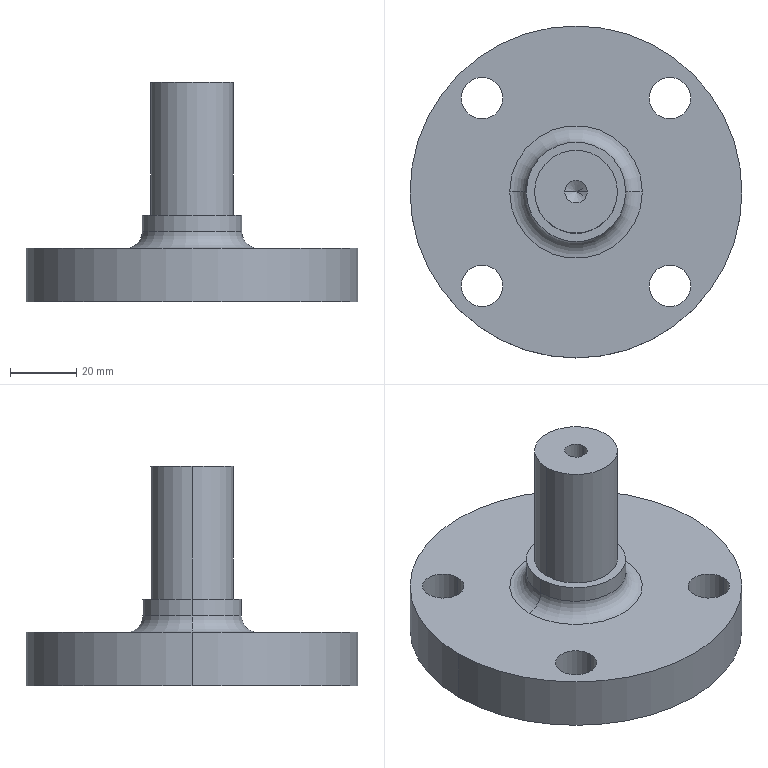Part | SolidWorks | features HoleWzd 2, ICE 2, CirPattern 1, Extrusion 1, Fillet 1 | 1 solid | 24 faces | box 100 x 100 x 66 mm | volume 144315 mm3 | cylinder 16 | plane 4 | torus 2 | cone 2 | commonest cylinder face diameters 12.5 x8 6.8 x2 25 x2 30 x2 100 x2
STEP:
#1=CARTESIAN_POINT('',(-15.,0.,21.));
#2=VERTEX_POINT('',#1);
#3=CARTESIAN_POINT('',(15.,0.,21.));
#4=VERTEX_POINT('',#3);
#5=CARTESIAN_POINT('',(0.,0.,21.));
#6=DIRECTION('',(0.,0.,1.));
#7=DIRECTION('',(1.,0.,0.));
#8=AXIS2_PLACEMENT_3D('',#5,#6,#7);
#9=CIRCLE('',#8,15.);
#10=EDGE_CURVE('',#2,#4,#9,.T.);
#11=ORIENTED_EDGE('',*,*,#10,.F.);
#12=CARTESIAN_POINT('',(-20.,0.,16.));
#13=VERTEX_POINT('',#12);
#14=CARTESIAN_POINT('',(-20.,0.,21.));
#15=DIRECTION('',(0.,1.,0.));
#16=DIRECTION('',(-1.,0.,0.));
#17=AXIS2_PLACEMENT_3D('',#14,#15,#16);
#18=CIRCLE('',#17,5.);
#19=EDGE_CURVE('',#2,#13,#18,.T.);
#20=ORIENTED_EDGE('',*,*,#19,.T.);
#21=CARTESIAN_POINT('',(20.,0.,16.));
#22=VERTEX_POINT('',#21);
#23=CARTESIAN_POINT('',(0.,0.,16.));
#24=DIRECTION('',(0.,0.,-1.));
#25=DIRECTION('',(1.,0.,0.));
#26=AXIS2_PLACEMENT_3D('',#23,#24,#25);
#27=CIRCLE('',#26,20.);
#28=EDGE_CURVE('',#22,#13,#27,.T.);
#29=ORIENTED_EDGE('',*,*,#28,.F.);
#30=CARTESIAN_POINT('',(20.,0.,21.));
#31=DIRECTION('',(0.,-1.,0.));
#32=DIRECTION('',(0.,0.,-1.));
#33=AXIS2_PLACEMENT_3D('',#30,#31,#32);
#34=CIRCLE('',#33,5.);
#35=EDGE_CURVE('',#4,#22,#34,.T.);
#36=ORIENTED_EDGE('',*,*,#35,.F.);
#37=EDGE_LOOP('',(#11,#20,#29,#36));
#38=FACE_OUTER_BOUND('',#37,.T.);
#39=CARTESIAN_POINT('',(0.,0.,21.));
#40=DIRECTION('',(0.,0.,1.));
#41=DIRECTION('',(1.,0.,0.));
#42=AXIS2_PLACEMENT_3D('',#39,#40,#41);
#43=TOROIDAL_SURFACE('',#42,20.,5.);
#44=ADVANCED_FACE('',(#38),#43,.F.);
#45=CARTESIAN_POINT('',(-3.4,0.,46.25));
#46=VERTEX_POINT('',#45);
#47=CARTESIAN_POINT('',(3.4,0.,46.25));
#48=VERTEX_POINT('',#47);
#49=CARTESIAN_POINT('',(0.,0.,46.25));
#50=DIRECTION('',(0.,0.,1.));
#51=DIRECTION('',(1.,0.,0.));
#52=AXIS2_PLACEMENT_3D('',#49,#50,#51);
#53=CIRCLE('',#52,3.4);
#54=EDGE_CURVE('',#46,#48,#53,.T.);
#55=ORIENTED_EDGE('',*,*,#54,.F.);
#56=CARTESIAN_POINT('',(-3.4,0.,66.));
#57=VERTEX_POINT('',#56);
#58=CARTESIAN_POINT('',(-3.4,0.,66.));
#59=DIRECTION('',(0.,0.,1.));
#60=VECTOR('',#59,1000.);
#61=LINE('',#58,#60);
#62=EDGE_CURVE('',#46,#57,#61,.T.);
#63=ORIENTED_EDGE('',*,*,#62,.T.);
#64=CARTESIAN_POINT('',(3.4,0.,66.));
#65=VERTEX_POINT('',#64);
#66=CARTESIAN_POINT('',(0.,0.,66.));
#67=DIRECTION('',(0.,0.,1.));
#68=DIRECTION('',(1.,0.,0.));
#69=AXIS2_PLACEMENT_3D('',#66,#67,#68);
#70=CIRCLE('',#69,3.4);
#71=EDGE_CURVE('',#57,#65,#70,.T.);
#72=ORIENTED_EDGE('',*,*,#71,.T.);
#73=CARTESIAN_POINT('',(3.4,0.,66.));
#74=DIRECTION('',(0.,0.,1.));
#75=VECTOR('',#74,1000.);
#76=LINE('',#73,#75);
#77=EDGE_CURVE('',#48,#65,#76,.T.);
#78=ORIENTED_EDGE('',*,*,#77,.F.);
#79=EDGE_LOOP('',(#55,#63,#72,#78));
#80=FACE_OUTER_BOUND('',#79,.T.);
#81=CARTESIAN_POINT('',(0.,0.,66.));
#82=DIRECTION('',(0.,0.,1.));
#83=DIRECTION('',(1.,0.,0.));
#84=AXIS2_PLACEMENT_3D('',#81,#82,#83);
#85=CYLINDRICAL_SURFACE('',#84,3.4);
#86=ADVANCED_FACE('',(#80),#85,.F.);
#87=CARTESIAN_POINT('',(0.,0.,44.207));
#88=VERTEX_POINT('',#87);
#89=CARTESIAN_POINT('',(3.4,0.,46.25));
#90=DIRECTION('',(0.8572,0.,0.515));
#91=VECTOR('',#90,1000.);
#92=LINE('',#89,#91);
#93=EDGE_CURVE('',#88,#48,#92,.T.);
#94=ORIENTED_EDGE('',*,*,#93,.F.);
#95=CARTESIAN_POINT('',(-3.4,0.,46.25));
#96=DIRECTION('',(-0.8572,0.,0.515));
#97=VECTOR('',#96,1000.);
#98=LINE('',#95,#97);
#99=EDGE_CURVE('',#88,#46,#98,.T.);
#100=ORIENTED_EDGE('',*,*,#99,.T.);
#101=ORIENTED_EDGE('',*,*,#54,.T.);
#102=EDGE_LOOP('',(#94,#100,#101));
#103=FACE_OUTER_BOUND('',#102,.T.);
#104=CARTESIAN_POINT('',(0.,0.,46.25));
#105=DIRECTION('',(0.,0.,1.));
#106=DIRECTION('',(1.,0.,0.));
#107=AXIS2_PLACEMENT_3D('',#104,#105,#106);
#108=CONICAL_SURFACE('',#107,3.4,1.03);
#109=ADVANCED_FACE('',(#103),#108,.F.);
#110=CARTESIAN_POINT('',(22.034,28.284,0.));
#111=VERTEX_POINT('',#110);
#112=CARTESIAN_POINT('',(34.534,28.284,0.));
#113=VERTEX_POINT('',#112);
#114=CARTESIAN_POINT('',(28.284,28.284,0.));
#115=DIRECTION('',(0.,0.,1.));
#116=DIRECTION('',(1.,0.,0.));
#117=AXIS2_PLACEMENT_3D('',#114,#115,#116);
#118=CIRCLE('',#117,6.25);
#119=EDGE_CURVE('',#111,#113,#118,.T.);
#120=ORIENTED_EDGE('',*,*,#119,.F.);
#121=CARTESIAN_POINT('',(22.034,28.284,16.));
#122=VERTEX_POINT('',#121);
#123=CARTESIAN_POINT('',(22.034,28.284,16.));
#124=DIRECTION('',(0.,0.,1.));
#125=VECTOR('',#124,1000.);
#126=LINE('',#123,#125);
#127=EDGE_CURVE('',#111,#122,#126,.T.);
#128=ORIENTED_EDGE('',*,*,#127,.T.);
#129=CARTESIAN_POINT('',(34.534,28.284,16.));
#130=VERTEX_POINT('',#129);
#131=CARTESIAN_POINT('',(28.284,28.284,16.));
#132=DIRECTION('',(0.,0.,1.));
#133=DIRECTION('',(1.,0.,0.));
#134=AXIS2_PLACEMENT_3D('',#131,#132,#133);
#135=CIRCLE('',#134,6.25);
#136=EDGE_CURVE('',#122,#130,#135,.T.);
#137=ORIENTED_EDGE('',*,*,#136,.T.);
#138=CARTESIAN_POINT('',(34.534,28.284,16.));
#139=DIRECTION('',(0.,0.,1.));
#140=VECTOR('',#139,1000.);
#141=LINE('',#138,#140);
#142=EDGE_CURVE('',#113,#130,#141,.T.);
#143=ORIENTED_EDGE('',*,*,#142,.F.);
#144=EDGE_LOOP('',(#120,#128,#137,#143));
#145=FACE_OUTER_BOUND('',#144,.T.);
#146=CARTESIAN_POINT('',(28.284,28.284,16.));
#147=DIRECTION('',(0.,0.,1.));
#148=DIRECTION('',(1.,0.,0.));
#149=AXIS2_PLACEMENT_3D('',#146,#147,#148);
#150=CYLINDRICAL_SURFACE('',#149,6.25);
#151=ADVANCED_FACE('',(#145),#150,.F.);
#152=CARTESIAN_POINT('',(22.034,-28.284,0.));
#153=VERTEX_POINT('',#152);
#154=CARTESIAN_POINT('',(34.534,-28.284,0.));
#155=VERTEX_POINT('',#154);
#156=CARTESIAN_POINT('',(28.284,-28.284,0.));
#157=DIRECTION('',(0.,0.,1.));
#158=DIRECTION('',(1.,0.,0.));
#159=AXIS2_PLACEMENT_3D('',#156,#157,#158);
#160=CIRCLE('',#159,6.25);
#161=EDGE_CURVE('',#153,#155,#160,.T.);
#162=ORIENTED_EDGE('',*,*,#161,.F.);
#163=CARTESIAN_POINT('',(22.034,-28.284,16.));
#164=VERTEX_POINT('',#163);
#165=CARTESIAN_POINT('',(22.034,-28.284,16.));
#166=DIRECTION('',(0.,0.,1.));
#167=VECTOR('',#166,1000.);
#168=LINE('',#165,#167);
#169=EDGE_CURVE('',#153,#164,#168,.T.);
#170=ORIENTED_EDGE('',*,*,#169,.T.);
#171=CARTESIAN_POINT('',(34.534,-28.284,16.));
#172=VERTEX_POINT('',#171);
#173=CARTESIAN_POINT('',(28.284,-28.284,16.));
#174=DIRECTION('',(0.,0.,1.));
#175=DIRECTION('',(1.,0.,0.));
#176=AXIS2_PLACEMENT_3D('',#173,#174,#175);
#177=CIRCLE('',#176,6.25);
#178=EDGE_CURVE('',#164,#172,#177,.T.);
#179=ORIENTED_EDGE('',*,*,#178,.T.);
#180=CARTESIAN_POINT('',(34.534,-28.284,16.));
#181=DIRECTION('',(0.,0.,1.));
#182=VECTOR('',#181,1000.);
#183=LINE('',#180,#182);
#184=EDGE_CURVE('',#155,#172,#183,.T.);
#185=ORIENTED_EDGE('',*,*,#184,.F.);
#186=EDGE_LOOP('',(#162,#170,#179,#185));
#187=FACE_OUTER_BOUND('',#186,.T.);
#188=CARTESIAN_POINT('',(28.284,-28.284,16.));
#189=DIRECTION('',(0.,0.,1.));
#190=DIRECTION('',(1.,0.,0.));
#191=AXIS2_PLACEMENT_3D('',#188,#189,#190);
#192=CYLINDRICAL_SURFACE('',#191,6.25);
#193=ADVANCED_FACE('',(#187),#192,.F.);
#194=CARTESIAN_POINT('',(-34.534,-28.284,0.));
#195=VERTEX_POINT('',#194);
#196=CARTESIAN_POINT('',(-22.034,-28.284,0.));
#197=VERTEX_POINT('',#196);
#198=CARTESIAN_POINT('',(-28.284,-28.284,0.));
#199=DIRECTION('',(0.,0.,1.));
#200=DIRECTION('',(1.,0.,0.));
#201=AXIS2_PLACEMENT_3D('',#198,#199,#200);
#202=CIRCLE('',#201,6.25);
#203=EDGE_CURVE('',#195,#197,#202,.T.);
#204=ORIENTED_EDGE('',*,*,#203,.F.);
#205=CARTESIAN_POINT('',(-34.534,-28.284,16.));
#206=VERTEX_POINT('',#205);
#207=CARTESIAN_POINT('',(-34.534,-28.284,16.));
#208=DIRECTION('',(0.,0.,1.));
#209=VECTOR('',#208,1000.);
#210=LINE('',#207,#209);
#211=EDGE_CURVE('',#195,#206,#210,.T.);
#212=ORIENTED_EDGE('',*,*,#211,.T.);
#213=CARTESIAN_POINT('',(-22.034,-28.284,16.));
#214=VERTEX_POINT('',#213);
#215=CARTESIAN_POINT('',(-28.284,-28.284,16.));
#216=DIRECTION('',(0.,0.,1.));
#217=DIRECTION('',(1.,0.,0.));
#218=AXIS2_PLACEMENT_3D('',#215,#216,#217);
#219=CIRCLE('',#218,6.25);
#220=EDGE_CURVE('',#206,#214,#219,.T.);
#221=ORIENTED_EDGE('',*,*,#220,.T.);
#222=CARTESIAN_POINT('',(-22.034,-28.284,16.));
#223=DIRECTION('',(0.,0.,1.));
#224=VECTOR('',#223,1000.);
#225=LINE('',#222,#224);
#226=EDGE_CURVE('',#197,#214,#225,.T.);
#227=ORIENTED_EDGE('',*,*,#226,.F.);
#228=EDGE_LOOP('',(#204,#212,#221,#227));
#229=FACE_OUTER_BOUND('',#228,.T.);
#230=CARTESIAN_POINT('',(-28.284,-28.284,16.));
#231=DIRECTION('',(0.,0.,1.));
#232=DIRECTION('',(1.,0.,0.));
#233=AXIS2_PLACEMENT_3D('',#230,#231,#232);
#234=CYLINDRICAL_SURFACE('',#233,6.25);
#235=ADVANCED_FACE('',(#229),#234,.F.);
#236=CARTESIAN_POINT('',(-34.534,28.284,0.));
#237=VERTEX_POINT('',#236);
#238=CARTESIAN_POINT('',(-22.034,28.284,0.));
#239=VERTEX_POINT('',#238);
#240=CARTESIAN_POINT('',(-28.284,28.284,0.));
#241=DIRECTION('',(0.,0.,1.));
#242=DIRECTION('',(1.,0.,0.));
#243=AXIS2_PLACEMENT_3D('',#240,#241,#242);
#244=CIRCLE('',#243,6.25);
#245=EDGE_CURVE('',#237,#239,#244,.T.);
#246=ORIENTED_EDGE('',*,*,#245,.F.);
#247=CARTESIAN_POINT('',(-34.534,28.284,16.));
#248=VERTEX_POINT('',#247);
#249=CARTESIAN_POINT('',(-34.534,28.284,16.));
#250=DIRECTION('',(0.,0.,1.));
#251=VECTOR('',#250,1000.);
#252=LINE('',#249,#251);
#253=EDGE_CURVE('',#237,#248,#252,.T.);
#254=ORIENTED_EDGE('',*,*,#253,.T.);
#255=CARTESIAN_POINT('',(-22.034,28.284,16.));
#256=VERTEX_POINT('',#255);
#257=CARTESIAN_POINT('',(-28.284,28.284,16.));
#258=DIRECTION('',(0.,0.,1.));
#259=DIRECTION('',(1.,0.,0.));
#260=AXIS2_PLACEMENT_3D('',#257,#258,#259);
#261=CIRCLE('',#260,6.25);
#262=EDGE_CURVE('',#248,#256,#261,.T.);
#263=ORIENTED_EDGE('',*,*,#262,.T.);
#264=CARTESIAN_POINT('',(-22.034,28.284,16.));
#265=DIRECTION('',(0.,0.,1.));
#266=VECTOR('',#265,1000.);
#267=LINE('',#264,#266);
#268=EDGE_CURVE('',#239,#256,#267,.T.);
#269=ORIENTED_EDGE('',*,*,#268,.F.);
#270=EDGE_LOOP('',(#246,#254,#263,#269));
#271=FACE_OUTER_BOUND('',#270,.T.);
#272=CARTESIAN_POINT('',(-28.284,28.284,16.));
#273=DIRECTION('',(0.,0.,1.));
#274=DIRECTION('',(1.,0.,0.));
#275=AXIS2_PLACEMENT_3D('',#272,#273,#274);
#276=CYLINDRICAL_SURFACE('',#275,6.25);
#277=ADVANCED_FACE('',(#271),#276,.F.);
#278=CARTESIAN_POINT('',(12.5,0.,66.));
#279=VERTEX_POINT('',#278);
#280=CARTESIAN_POINT('',(-12.5,0.,66.));
#281=VERTEX_POINT('',#280);
#282=CARTESIAN_POINT('',(0.,0.,66.));
#283=DIRECTION('',(0.,0.,1.));
#284=DIRECTION('',(1.,0.,0.));
#285=AXIS2_PLACEMENT_3D('',#282,#283,#284);
#286=CIRCLE('',#285,12.5);
#287=EDGE_CURVE('',#279,#281,#286,.T.);
#288=ORIENTED_EDGE('',*,*,#287,.F.);
#289=CARTESIAN_POINT('',(12.5,0.,26.));
#290=VERTEX_POINT('',#289);
#291=CARTESIAN_POINT('',(12.5,0.,66.));
#292=DIRECTION('',(0.,0.,-1.));
#293=VECTOR('',#292,1000.);
#294=LINE('',#291,#293);
#295=EDGE_CURVE('',#279,#290,#294,.T.);
#296=ORIENTED_EDGE('',*,*,#295,.T.);
#297=CARTESIAN_POINT('',(-12.5,0.,26.));
#298=VERTEX_POINT('',#297);
#299=CARTESIAN_POINT('',(0.,0.,26.));
#300=DIRECTION('',(0.,0.,1.));
#301=DIRECTION('',(1.,0.,0.));
#302=AXIS2_PLACEMENT_3D('',#299,#300,#301);
#303=CIRCLE('',#302,12.5);
#304=EDGE_CURVE('',#290,#298,#303,.T.);
#305=ORIENTED_EDGE('',*,*,#304,.T.);
#306=CARTESIAN_POINT('',(-12.5,0.,66.));
#307=DIRECTION('',(0.,0.,-1.));
#308=VECTOR('',#307,1000.);
#309=LINE('',#306,#308);
#310=EDGE_CURVE('',#281,#298,#309,.T.);
#311=ORIENTED_EDGE('',*,*,#310,.F.);
#312=EDGE_LOOP('',(#288,#296,#305,#311));
#313=FACE_OUTER_BOUND('',#312,.T.);
#314=CARTESIAN_POINT('',(0.,0.,66.));
#315=DIRECTION('',(0.,0.,-1.));
#316=DIRECTION('',(-1.,0.,0.));
#317=AXIS2_PLACEMENT_3D('',#314,#315,#316);
#318=CYLINDRICAL_SURFACE('',#317,12.5);
#319=ADVANCED_FACE('',(#313),#318,.T.);
#320=CARTESIAN_POINT('',(15.,0.,26.));
#321=VERTEX_POINT('',#320);
#322=CARTESIAN_POINT('',(-15.,0.,26.));
#323=VERTEX_POINT('',#322);
#324=CARTESIAN_POINT('',(0.,0.,26.));
#325=DIRECTION('',(0.,0.,1.));
#326=DIRECTION('',(1.,0.,0.));
#327=AXIS2_PLACEMENT_3D('',#324,#325,#326);
#328=CIRCLE('',#327,15.);
#329=EDGE_CURVE('',#321,#323,#328,.T.);
#330=ORIENTED_EDGE('',*,*,#329,.F.);
#331=CARTESIAN_POINT('',(15.,0.,26.));
#332=DIRECTION('',(0.,0.,-1.));
#333=VECTOR('',#332,1000.);
#334=LINE('',#331,#333);
#335=EDGE_CURVE('',#321,#4,#334,.T.);
#336=ORIENTED_EDGE('',*,*,#335,.T.);
#337=CARTESIAN_POINT('',(0.,0.,21.));
#338=DIRECTION('',(0.,0.,1.));
#339=DIRECTION('',(1.,0.,0.));
#340=AXIS2_PLACEMENT_3D('',#337,#338,#339);
#341=CIRCLE('',#340,15.);
#342=EDGE_CURVE('',#4,#2,#341,.T.);
#343=ORIENTED_EDGE('',*,*,#342,.T.);
#344=CARTESIAN_POINT('',(-15.,0.,26.));
#345=DIRECTION('',(0.,0.,-1.));
#346=VECTOR('',#345,1000.);
#347=LINE('',#344,#346);
#348=EDGE_CURVE('',#323,#2,#347,.T.);
#349=ORIENTED_EDGE('',*,*,#348,.F.);
#350=EDGE_LOOP('',(#330,#336,#343,#349));
#351=FACE_OUTER_BOUND('',#350,.T.);
#352=CARTESIAN_POINT('',(0.,0.,26.));
#353=DIRECTION('',(0.,0.,-1.));
#354=DIRECTION('',(-1.,0.,0.));
#355=AXIS2_PLACEMENT_3D('',#352,#353,#354);
#356=CYLINDRICAL_SURFACE('',#355,15.);
#357=ADVANCED_FACE('',(#351),#356,.T.);
#358=CARTESIAN_POINT('',(50.,0.,16.));
#359=VERTEX_POINT('',#358);
#360=CARTESIAN_POINT('',(-50.,0.,16.));
#361=VERTEX_POINT('',#360);
#362=CARTESIAN_POINT('',(0.,0.,16.));
#363=DIRECTION('',(0.,0.,1.));
#364=DIRECTION('',(1.,0.,0.));
#365=AXIS2_PLACEMENT_3D('',#362,#363,#364);
#366=CIRCLE('',#365,50.);
#367=EDGE_CURVE('',#359,#361,#366,.T.);
#368=ORIENTED_EDGE('',*,*,#367,.F.);
#369=CARTESIAN_POINT('',(50.,0.,0.));
#370=VERTEX_POINT('',#369);
#371=CARTESIAN_POINT('',(50.,0.,16.));
#372=DIRECTION('',(0.,0.,-1.));
#373=VECTOR('',#372,1000.);
#374=LINE('',#371,#373);
#375=EDGE_CURVE('',#359,#370,#374,.T.);
#376=ORIENTED_EDGE('',*,*,#375,.T.);
#377=CARTESIAN_POINT('',(-50.,0.,0.));
#378=VERTEX_POINT('',#377);
#379=CARTESIAN_POINT('',(0.,0.,0.));
#380=DIRECTION('',(0.,0.,1.));
#381=DIRECTION('',(1.,0.,0.));
#382=AXIS2_PLACEMENT_3D('',#379,#380,#381);
#383=CIRCLE('',#382,50.);
#384=EDGE_CURVE('',#370,#378,#383,.T.);
#385=ORIENTED_EDGE('',*,*,#384,.T.);
#386=CARTESIAN_POINT('',(-50.,0.,16.));
#387=DIRECTION('',(0.,0.,-1.));
#388=VECTOR('',#387,1000.);
#389=LINE('',#386,#388);
#390=EDGE_CURVE('',#361,#378,#389,.T.);
#391=ORIENTED_EDGE('',*,*,#390,.F.);
#392=EDGE_LOOP('',(#368,#376,#385,#391));
#393=FACE_OUTER_BOUND('',#392,.T.);
#394=CARTESIAN_POINT('',(0.,0.,16.));
#395=DIRECTION('',(0.,0.,-1.));
#396=DIRECTION('',(-1.,0.,0.));
#397=AXIS2_PLACEMENT_3D('',#394,#395,#396);
#398=CYLINDRICAL_SURFACE('',#397,50.);
#399=ADVANCED_FACE('',(#393),#398,.T.);
#400=ORIENTED_EDGE('',*,*,#375,.F.);
#401=CARTESIAN_POINT('',(0.,0.,16.));
#402=DIRECTION('',(0.,0.,1.));
#403=DIRECTION('',(1.,0.,0.));
#404=AXIS2_PLACEMENT_3D('',#401,#402,#403);
#405=CIRCLE('',#404,50.);
#406=EDGE_CURVE('',#361,#359,#405,.T.);
#407=ORIENTED_EDGE('',*,*,#406,.F.);
#408=ORIENTED_EDGE('',*,*,#390,.T.);
#409=CARTESIAN_POINT('',(0.,0.,0.));
#410=DIRECTION('',(0.,0.,1.));
#411=DIRECTION('',(1.,0.,0.));
#412=AXIS2_PLACEMENT_3D('',#409,#410,#411);
#413=CIRCLE('',#412,50.);
#414=EDGE_CURVE('',#378,#370,#413,.T.);
#415=ORIENTED_EDGE('',*,*,#414,.T.);
#416=EDGE_LOOP('',(#400,#407,#408,#415));
#417=FACE_OUTER_BOUND('',#416,.T.);
#418=CARTESIAN_POINT('',(0.,0.,16.));
#419=DIRECTION('',(0.,0.,-1.));
#420=DIRECTION('',(-1.,0.,0.));
#421=AXIS2_PLACEMENT_3D('',#418,#419,#420);
#422=CYLINDRICAL_SURFACE('',#421,50.);
#423=ADVANCED_FACE('',(#417),#422,.T.);
#424=ORIENTED_EDGE('',*,*,#28,.T.);
#425=CARTESIAN_POINT('',(0.,0.,16.));
#426=DIRECTION('',(0.,0.,-1.));
#427=DIRECTION('',(1.,0.,0.));
#428=AXIS2_PLACEMENT_3D('',#425,#426,#427);
#429=CIRCLE('',#428,20.);
#430=EDGE_CURVE('',#13,#22,#429,.T.);
#431=ORIENTED_EDGE('',*,*,#430,.T.);
#432=EDGE_LOOP('',(#424,#431));
#433=FACE_BOUND('',#432,.T.);
#434=CARTESIAN_POINT('',(28.284,28.284,16.));
#435=DIRECTION('',(0.,0.,1.));
#436=DIRECTION('',(1.,0.,0.));
#437=AXIS2_PLACEMENT_3D('',#434,#435,#436);
#438=CIRCLE('',#437,6.25);
#439=EDGE_CURVE('',#130,#122,#438,.T.);
#440=ORIENTED_EDGE('',*,*,#439,.F.);
#441=ORIENTED_EDGE('',*,*,#136,.F.);
#442=EDGE_LOOP('',(#440,#441));
#443=FACE_BOUND('',#442,.T.);
#444=CARTESIAN_POINT('',(28.284,-28.284,16.));
#445=DIRECTION('',(0.,0.,1.));
#446=DIRECTION('',(1.,0.,0.));
#447=AXIS2_PLACEMENT_3D('',#444,#445,#446);
#448=CIRCLE('',#447,6.25);
#449=EDGE_CURVE('',#172,#164,#448,.T.);
#450=ORIENTED_EDGE('',*,*,#449,.F.);
#451=ORIENTED_EDGE('',*,*,#178,.F.);
#452=EDGE_LOOP('',(#450,#451));
#453=FACE_BOUND('',#452,.T.);
#454=CARTESIAN_POINT('',(-28.284,-28.284,16.));
#455=DIRECTION('',(0.,0.,1.));
#456=DIRECTION('',(1.,0.,0.));
#457=AXIS2_PLACEMENT_3D('',#454,#455,#456);
#458=CIRCLE('',#457,6.25);
#459=EDGE_CURVE('',#214,#206,#458,.T.);
#460=ORIENTED_EDGE('',*,*,#459,.F.);
#461=ORIENTED_EDGE('',*,*,#220,.F.);
#462=EDGE_LOOP('',(#460,#461));
#463=FACE_BOUND('',#462,.T.);
#464=CARTESIAN_POINT('',(-28.284,28.284,16.));
#465=DIRECTION('',(0.,0.,1.));
#466=DIRECTION('',(1.,0.,0.));
#467=AXIS2_PLACEMENT_3D('',#464,#465,#466);
#468=CIRCLE('',#467,6.25);
#469=EDGE_CURVE('',#256,#248,#468,.T.);
#470=ORIENTED_EDGE('',*,*,#469,.F.);
#471=ORIENTED_EDGE('',*,*,#262,.F.);
#472=EDGE_LOOP('',(#470,#471));
#473=FACE_BOUND('',#472,.T.);
#474=ORIENTED_EDGE('',*,*,#406,.T.);
#475=ORIENTED_EDGE('',*,*,#367,.T.);
#476=EDGE_LOOP('',(#474,#475));
#477=FACE_OUTER_BOUND('',#476,.T.);
#478=CARTESIAN_POINT('',(0.,0.,16.));
#479=DIRECTION('',(0.,0.,1.));
#480=DIRECTION('',(1.,0.,0.));
#481=AXIS2_PLACEMENT_3D('',#478,#479,#480);
#482=PLANE('',#481);
#483=ADVANCED_FACE('',(#433,#443,#453,#463,#473,#477),#482,.T.);
#484=CARTESIAN_POINT('',(28.284,28.284,0.));
#485=DIRECTION('',(0.,0.,1.));
#486=DIRECTION('',(1.,0.,0.));
#487=AXIS2_PLACEMENT_3D('',#484,#485,#486);
#488=CIRCLE('',#487,6.25);
#489=EDGE_CURVE('',#113,#111,#488,.T.);
#490=ORIENTED_EDGE('',*,*,#489,.T.);
#491=ORIENTED_EDGE('',*,*,#119,.T.);
#492=EDGE_LOOP('',(#490,#491));
#493=FACE_BOUND('',#492,.T.);
#494=CARTESIAN_POINT('',(28.284,-28.284,0.));
#495=DIRECTION('',(0.,0.,1.));
#496=DIRECTION('',(1.,0.,0.));
#497=AXIS2_PLACEMENT_3D('',#494,#495,#496);
#498=CIRCLE('',#497,6.25);
#499=EDGE_CURVE('',#155,#153,#498,.T.);
#500=ORIENTED_EDGE('',*,*,#499,.T.);
#501=ORIENTED_EDGE('',*,*,#161,.T.);
#502=EDGE_LOOP('',(#500,#501));
#503=FACE_BOUND('',#502,.T.);
#504=CARTESIAN_POINT('',(-28.284,-28.284,0.));
#505=DIRECTION('',(0.,0.,1.));
#506=DIRECTION('',(1.,0.,0.));
#507=AXIS2_PLACEMENT_3D('',#504,#505,#506);
#508=CIRCLE('',#507,6.25);
#509=EDGE_CURVE('',#197,#195,#508,.T.);
#510=ORIENTED_EDGE('',*,*,#509,.T.);
#511=ORIENTED_EDGE('',*,*,#203,.T.);
#512=EDGE_LOOP('',(#510,#511));
#513=FACE_BOUND('',#512,.T.);
#514=CARTESIAN_POINT('',(-28.284,28.284,0.));
#515=DIRECTION('',(0.,0.,1.));
#516=DIRECTION('',(1.,0.,0.));
#517=AXIS2_PLACEMENT_3D('',#514,#515,#516);
#518=CIRCLE('',#517,6.25);
#519=EDGE_CURVE('',#239,#237,#518,.T.);
#520=ORIENTED_EDGE('',*,*,#519,.T.);
#521=ORIENTED_EDGE('',*,*,#245,.T.);
#522=EDGE_LOOP('',(#520,#521));
#523=FACE_BOUND('',#522,.T.);
#524=ORIENTED_EDGE('',*,*,#414,.F.);
#525=ORIENTED_EDGE('',*,*,#384,.F.);
#526=EDGE_LOOP('',(#524,#525));
#527=FACE_OUTER_BOUND('',#526,.T.);
#528=CARTESIAN_POINT('',(0.,0.,0.));
#529=DIRECTION('',(0.,0.,1.));
#530=DIRECTION('',(1.,0.,0.));
#531=AXIS2_PLACEMENT_3D('',#528,#529,#530);
#532=PLANE('',#531);
#533=ADVANCED_FACE('',(#493,#503,#513,#523,#527),#532,.F.);
#534=ORIENTED_EDGE('',*,*,#335,.F.);
#535=CARTESIAN_POINT('',(0.,0.,26.));
#536=DIRECTION('',(0.,0.,1.));
#537=DIRECTION('',(1.,0.,0.));
#538=AXIS2_PLACEMENT_3D('',#535,#536,#537);
#539=CIRCLE('',#538,15.);
#540=EDGE_CURVE('',#323,#321,#539,.T.);
#541=ORIENTED_EDGE('',*,*,#540,.F.);
#542=ORIENTED_EDGE('',*,*,#348,.T.);
#543=ORIENTED_EDGE('',*,*,#10,.T.);
#544=EDGE_LOOP('',(#534,#541,#542,#543));
#545=FACE_OUTER_BOUND('',#544,.T.);
#546=CARTESIAN_POINT('',(0.,0.,26.));
#547=DIRECTION('',(0.,0.,-1.));
#548=DIRECTION('',(-1.,0.,0.));
#549=AXIS2_PLACEMENT_3D('',#546,#547,#548);
#550=CYLINDRICAL_SURFACE('',#549,15.);
#551=ADVANCED_FACE('',(#545),#550,.T.);
#552=CARTESIAN_POINT('',(0.,0.,26.));
#553=DIRECTION('',(0.,0.,1.));
#554=DIRECTION('',(1.,0.,0.));
#555=AXIS2_PLACEMENT_3D('',#552,#553,#554);
#556=CIRCLE('',#555,12.5);
#557=EDGE_CURVE('',#298,#290,#556,.T.);
#558=ORIENTED_EDGE('',*,*,#557,.F.);
#559=ORIENTED_EDGE('',*,*,#304,.F.);
#560=EDGE_LOOP('',(#558,#559));
#561=FACE_BOUND('',#560,.T.);
#562=ORIENTED_EDGE('',*,*,#540,.T.);
#563=ORIENTED_EDGE('',*,*,#329,.T.);
#564=EDGE_LOOP('',(#562,#563));
#565=FACE_OUTER_BOUND('',#564,.T.);
#566=CARTESIAN_POINT('',(0.,0.,26.));
#567=DIRECTION('',(0.,0.,1.));
#568=DIRECTION('',(1.,0.,0.));
#569=AXIS2_PLACEMENT_3D('',#566,#567,#568);
#570=PLANE('',#569);
#571=ADVANCED_FACE('',(#561,#565),#570,.T.);
#572=ORIENTED_EDGE('',*,*,#295,.F.);
#573=CARTESIAN_POINT('',(0.,0.,66.));
#574=DIRECTION('',(0.,0.,1.));
#575=DIRECTION('',(1.,0.,0.));
#576=AXIS2_PLACEMENT_3D('',#573,#574,#575);
#577=CIRCLE('',#576,12.5);
#578=EDGE_CURVE('',#281,#279,#577,.T.);
#579=ORIENTED_EDGE('',*,*,#578,.F.);
#580=ORIENTED_EDGE('',*,*,#310,.T.);
#581=ORIENTED_EDGE('',*,*,#557,.T.);
#582=EDGE_LOOP('',(#572,#579,#580,#581));
#583=FACE_OUTER_BOUND('',#582,.T.);
#584=CARTESIAN_POINT('',(0.,0.,66.));
#585=DIRECTION('',(0.,0.,-1.));
#586=DIRECTION('',(-1.,0.,0.));
#587=AXIS2_PLACEMENT_3D('',#584,#585,#586);
#588=CYLINDRICAL_SURFACE('',#587,12.5);
#589=ADVANCED_FACE('',(#583),#588,.T.);
#590=CARTESIAN_POINT('',(0.,0.,66.));
#591=DIRECTION('',(0.,0.,1.));
#592=DIRECTION('',(1.,0.,0.));
#593=AXIS2_PLACEMENT_3D('',#590,#591,#592);
#594=CIRCLE('',#593,3.4);
#595=EDGE_CURVE('',#65,#57,#594,.T.);
#596=ORIENTED_EDGE('',*,*,#595,.F.);
#597=ORIENTED_EDGE('',*,*,#71,.F.);
#598=EDGE_LOOP('',(#596,#597));
#599=FACE_BOUND('',#598,.T.);
#600=ORIENTED_EDGE('',*,*,#578,.T.);
#601=ORIENTED_EDGE('',*,*,#287,.T.);
#602=EDGE_LOOP('',(#600,#601));
#603=FACE_OUTER_BOUND('',#602,.T.);
#604=CARTESIAN_POINT('',(0.,0.,66.));
#605=DIRECTION('',(0.,0.,1.));
#606=DIRECTION('',(1.,0.,0.));
#607=AXIS2_PLACEMENT_3D('',#604,#605,#606);
#608=PLANE('',#607);
#609=ADVANCED_FACE('',(#599,#603),#608,.T.);
#610=ORIENTED_EDGE('',*,*,#253,.F.);
#611=ORIENTED_EDGE('',*,*,#519,.F.);
#612=ORIENTED_EDGE('',*,*,#268,.T.);
#613=ORIENTED_EDGE('',*,*,#469,.T.);
#614=EDGE_LOOP('',(#610,#611,#612,#613));
#615=FACE_OUTER_BOUND('',#614,.T.);
#616=CARTESIAN_POINT('',(-28.284,28.284,16.));
#617=DIRECTION('',(0.,0.,1.));
#618=DIRECTION('',(1.,0.,0.));
#619=AXIS2_PLACEMENT_3D('',#616,#617,#618);
#620=CYLINDRICAL_SURFACE('',#619,6.25);
#621=ADVANCED_FACE('',(#615),#620,.F.);
#622=ORIENTED_EDGE('',*,*,#211,.F.);
#623=ORIENTED_EDGE('',*,*,#509,.F.);
#624=ORIENTED_EDGE('',*,*,#226,.T.);
#625=ORIENTED_EDGE('',*,*,#459,.T.);
#626=EDGE_LOOP('',(#622,#623,#624,#625));
#627=FACE_OUTER_BOUND('',#626,.T.);
#628=CARTESIAN_POINT('',(-28.284,-28.284,16.));
#629=DIRECTION('',(0.,0.,1.));
#630=DIRECTION('',(1.,0.,0.));
#631=AXIS2_PLACEMENT_3D('',#628,#629,#630);
#632=CYLINDRICAL_SURFACE('',#631,6.25);
#633=ADVANCED_FACE('',(#627),#632,.F.);
#634=ORIENTED_EDGE('',*,*,#169,.F.);
#635=ORIENTED_EDGE('',*,*,#499,.F.);
#636=ORIENTED_EDGE('',*,*,#184,.T.);
#637=ORIENTED_EDGE('',*,*,#449,.T.);
#638=EDGE_LOOP('',(#634,#635,#636,#637));
#639=FACE_OUTER_BOUND('',#638,.T.);
#640=CARTESIAN_POINT('',(28.284,-28.284,16.));
#641=DIRECTION('',(0.,0.,1.));
#642=DIRECTION('',(1.,0.,0.));
#643=AXIS2_PLACEMENT_3D('',#640,#641,#642);
#644=CYLINDRICAL_SURFACE('',#643,6.25);
#645=ADVANCED_FACE('',(#639),#644,.F.);
#646=ORIENTED_EDGE('',*,*,#127,.F.);
#647=ORIENTED_EDGE('',*,*,#489,.F.);
#648=ORIENTED_EDGE('',*,*,#142,.T.);
#649=ORIENTED_EDGE('',*,*,#439,.T.);
#650=EDGE_LOOP('',(#646,#647,#648,#649));
#651=FACE_OUTER_BOUND('',#650,.T.);
#652=CARTESIAN_POINT('',(28.284,28.284,16.));
#653=DIRECTION('',(0.,0.,1.));
#654=DIRECTION('',(1.,0.,0.));
#655=AXIS2_PLACEMENT_3D('',#652,#653,#654);
#656=CYLINDRICAL_SURFACE('',#655,6.25);
#657=ADVANCED_FACE('',(#651),#656,.F.);
#658=ORIENTED_EDGE('',*,*,#99,.F.);
#659=ORIENTED_EDGE('',*,*,#93,.T.);
#660=CARTESIAN_POINT('',(0.,0.,46.25));
#661=DIRECTION('',(0.,0.,1.));
#662=DIRECTION('',(1.,0.,0.));
#663=AXIS2_PLACEMENT_3D('',#660,#661,#662);
#664=CIRCLE('',#663,3.4);
#665=EDGE_CURVE('',#48,#46,#664,.T.);
#666=ORIENTED_EDGE('',*,*,#665,.T.);
#667=EDGE_LOOP('',(#658,#659,#666));
#668=FACE_OUTER_BOUND('',#667,.T.);
#669=CARTESIAN_POINT('',(0.,0.,46.25));
#670=DIRECTION('',(0.,0.,1.));
#671=DIRECTION('',(1.,0.,0.));
#672=AXIS2_PLACEMENT_3D('',#669,#670,#671);
#673=CONICAL_SURFACE('',#672,3.4,1.03);
#674=ADVANCED_FACE('',(#668),#673,.F.);
#675=ORIENTED_EDGE('',*,*,#62,.F.);
#676=ORIENTED_EDGE('',*,*,#665,.F.);
#677=ORIENTED_EDGE('',*,*,#77,.T.);
#678=ORIENTED_EDGE('',*,*,#595,.T.);
#679=EDGE_LOOP('',(#675,#676,#677,#678));
#680=FACE_OUTER_BOUND('',#679,.T.);
#681=CARTESIAN_POINT('',(0.,0.,66.));
#682=DIRECTION('',(0.,0.,1.));
#683=DIRECTION('',(1.,0.,0.));
#684=AXIS2_PLACEMENT_3D('',#681,#682,#683);
#685=CYLINDRICAL_SURFACE('',#684,3.4);
#686=ADVANCED_FACE('',(#680),#685,.F.);
#687=ORIENTED_EDGE('',*,*,#19,.F.);
#688=ORIENTED_EDGE('',*,*,#342,.F.);
#689=ORIENTED_EDGE('',*,*,#35,.T.);
#690=ORIENTED_EDGE('',*,*,#430,.F.);
#691=EDGE_LOOP('',(#687,#688,#689,#690));
#692=FACE_OUTER_BOUND('',#691,.T.);
#693=CARTESIAN_POINT('',(0.,0.,21.));
#694=DIRECTION('',(0.,0.,1.));
#695=DIRECTION('',(1.,0.,0.));
#696=AXIS2_PLACEMENT_3D('',#693,#694,#695);
#697=TOROIDAL_SURFACE('',#696,20.,5.);
#698=ADVANCED_FACE('',(#692),#697,.F.);
#699=CLOSED_SHELL('',(#44,#86,#109,#151,#193,#235,#277,#319,#357,#399,#423,#483,#533,#551,#571,#589,#609,#621,#633,#645,#657,#674,#686,#698));
#700=MANIFOLD_SOLID_BREP('',#699);
#701=CARTESIAN_POINT('',(0.,0.,0.));
#702=DIRECTION('',(0.,0.,1.));
#703=DIRECTION('',(1.,0.,0.));
#704=AXIS2_PLACEMENT_3D('',#701,#702,#703);
#705=(LENGTH_UNIT()NAMED_UNIT(*)SI_UNIT(.MILLI.,.METRE.));
#706=UNCERTAINTY_MEASURE_WITH_UNIT(LENGTH_MEASURE(0.00001),#705,'','');
#707=(NAMED_UNIT(*)PLANE_ANGLE_UNIT()SI_UNIT($,.RADIAN.));
#708=(NAMED_UNIT(*)SI_UNIT($,.STERADIAN.)SOLID_ANGLE_UNIT());
#709=(GEOMETRIC_REPRESENTATION_CONTEXT(3)GLOBAL_UNCERTAINTY_ASSIGNED_CONTEXT((#706))GLOBAL_UNIT_ASSIGNED_CONTEXT((#705,#707,#708))REPRESENTATION_CONTEXT('',''));
#710=ADVANCED_BREP_SHAPE_REPRESENTATION('',(#700,#704),#709);